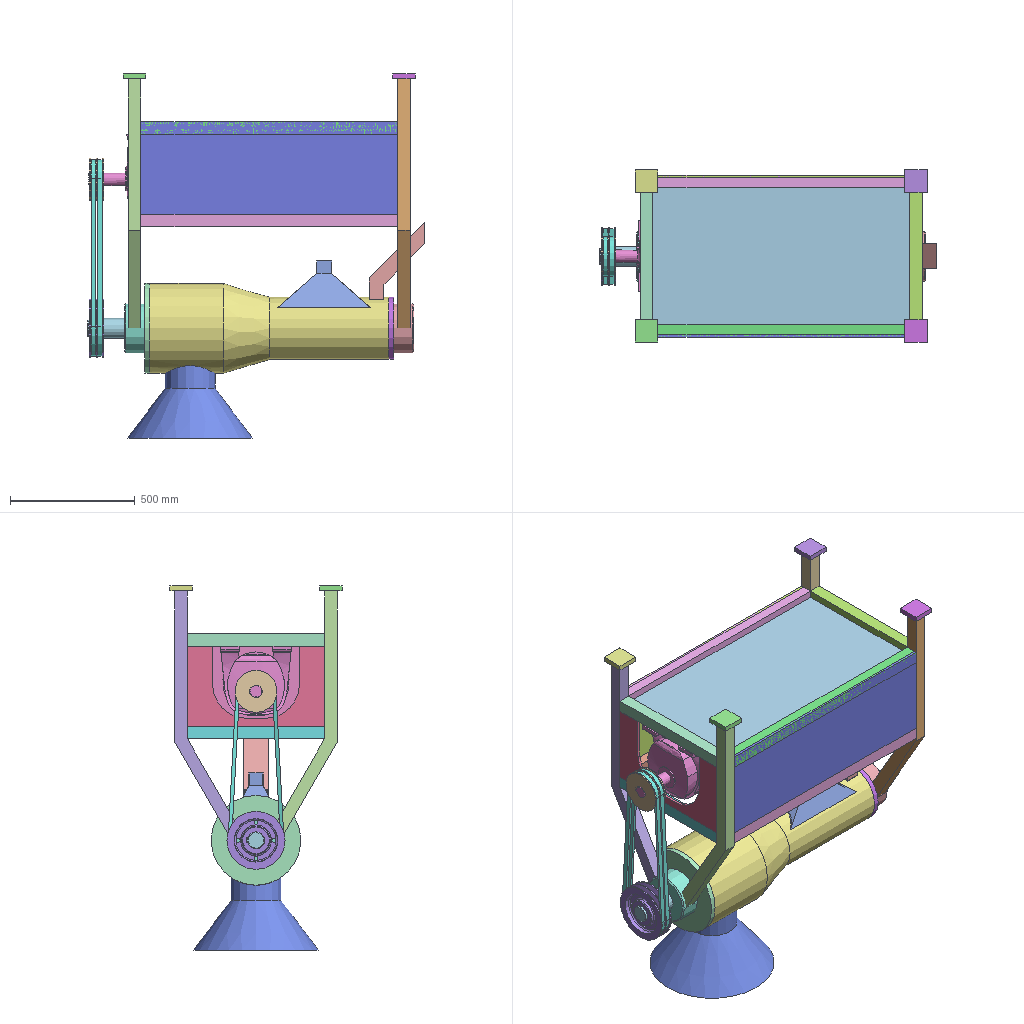Assembly | NX | 16 different items | 17 placed | box 1349 x 690 x 1460 mm
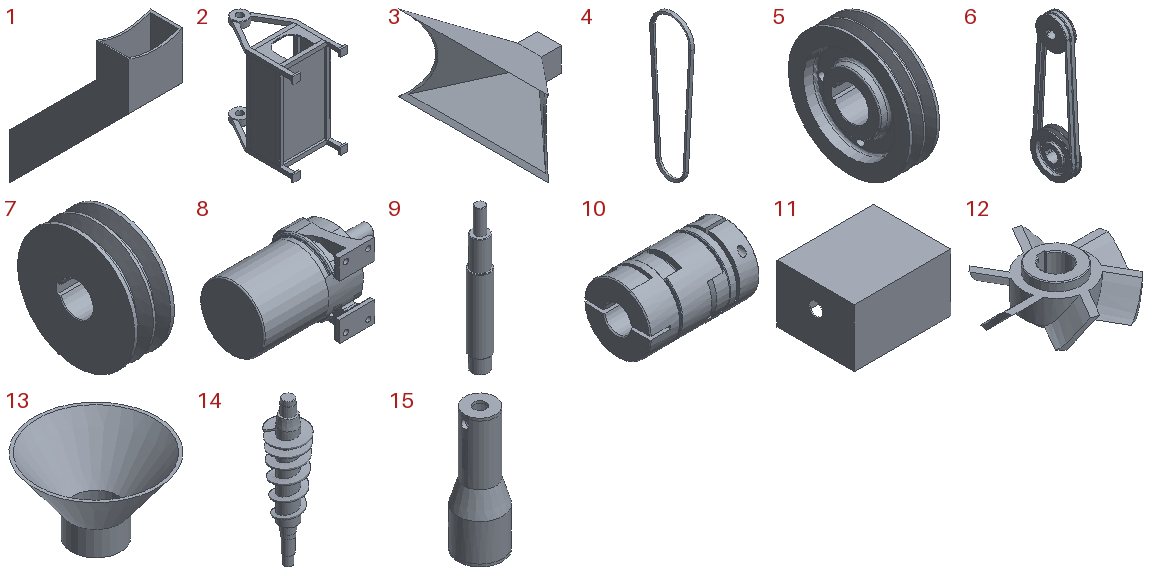Parts list (item | name | quantity | parent item | size | volume | features):
1 | - | x1 | - | 100 x 220.919 x 308.781 mm | 414084 mm3 | features DATUM_CSYS 3, EXTRUDE 2, SKETCH 2, CHAMFER 1, SHELL 1
2 | - | x1 | - | 690 x 1120 x 1170 mm | 52680048 mm3 | features DATUM_CSYS 11, EXTRUDE 10, SKETCH 10, EXTRACT_BODY 8, Container 2, Geometry Instance 2, LINKED_FACE 2, CHAMFER 1, CYLINDER 1, LINKED_CURVE 1
3 | - | x1 | - | 188.137 x 373.11 x 188.928 mm | 418507 mm3 | features NSIDED_SURFACE 6, DATUM_CSYS 5, LINE 4, SKETCH 3, EXTRUDE 2, SEW 1, SHELL 1
4 | - | x2 | in 6 | 19 x 224 x 789.47 mm | 368031 mm3 | features sk_皮带 2
5 | - | x1 | in 6 | 57.5 x 233.6 x 233.6 mm | 1208197 mm3 | features 大带轮_孔板轮(A) 2
6 | - | x1 | - | 57.5 x 233.6 x 799.07 mm | 2816875 mm3 | features sk_皮带 2, 大带轮_孔板轮(A) 2, 小带轮_实心轮 2
7 | - | x1 | in 6 | 57.5 x 169.6 x 169.6 mm | 872615 mm3 | features 小带轮_实心轮 2
8 | - | x1 | - | 553.467 x 279.469 x 285.867 mm | 20300035 mm3 | features BREP 1
9 | - | x1 | - | 80 x 80 x 580 mm | 2266189 mm3 | features CYLINDER 4, CHAMFER 1, DATUM_CSYS 1
10 | - | x1 | - | 165 x 100 x 100 mm | 960558 mm3 | features BREP 5
11 | - | x1 | - | 500 x 400 x 300 mm | 3606133 mm3 | features DATUM_CSYS 2, BLOCK 1, EXTRUDE 1, SHELL 1, SKETCH 1
12 | - | x1 | - | 300.002 x 290.157 x 100 mm | 1656356 mm3 | features DATUM_CSYS 7, EXTRUDE 7, EXTRACT_BODY 6, SKETCH 6, BLEND 2, CHAMFER 1, Container 1, Geometry Instance 1, HOLE PACKAGE 1, SIMPLE HOLE 1, UNITE 1
13 | - | x1 | - | 500 x 500 x 300 mm | 3245287 mm3 | features CONE 1, CYLINDER 1, DATUM_CSYS 1, SHELL 1
14 | - | x1 | - | 177.285 x 178.372 x 728 mm | 4210187 mm3 | features CYLINDER 7, DATUM_CSYS 4, CHAMFER 2, SKETCH 2, UNITE 2, EXTRUDE 1, HELIX 1, LINE 1, SKIN 1
15 | - | x1 | - | 360 x 360 x 1000 mm | 21575281 mm3 | features CYLINDER 4, DATUM_CSYS 4, EXTRUDE 3, SKETCH 3, SPLIT BODY 2, CHAMFER 1, SHELL 1
16 | Fruit Pulper General Assembly | x1 | - | - | - | -
Mates (type | each side: item.copy, entity, surface, feature):
Touch | 12.1 face cylinder Ø67 Hole(14) | 5.1 face cylinder Large Pulley_Web Plate Wheel(A)(1)
Touch | 14.1 face cylinder Cylinder(2) | 12.1 face cylinder Extrude(13)
Touch | 15.1 face cylinder Cylinder(1) | 14.1 face cylinder Cylinder(7)
Distance | 15.1 face plane Cylinder(1) | 14.1 face plane Cylinder(4)
Touch | 9.1 face cylinder Cylinder(2) | 5.1 face cylinder Large Pulley_Web Plate Wheel(A)(1)
Distance | 9.1 face plane Cylinder(3) | 5.1 face plane Large Pulley_Web Plate Wheel(A)(1)
Touch | 10.1 face cylinder Body(0) | 9.1 face cylinder Cylinder(5)
Distance | 10.1 face plane Body(0) | 14.1 face plane Cylinder(2)
Distance | 12.1 face plane Extrude(1) | 9.1 face plane Cylinder(3)
Distance | 8.1 face plane Body(0) | 7.1 face plane Small Pulley_Solid Wheel(1)
Touch | 7.1 face cylinder Small Pulley_Solid Wheel(1) | 8.1 face cylinder Body(0)
Touch | 2.1 face plane Extrude(2) | 15.1 face plane Cylinder(2)
Touch | 2.1 face cylinder Cylinder(3) | 9.1 face cylinder Cylinder(3)
Center12 | 12.1 face plane Extrude(1) | 12.1 face plane Extrude(1) | 13.1 face cylinder Shell(4)
Distance | 13.1 face plane Cylinder(2) | 12.1 face cylinder Ø67 Hole(14)
Center12 | 3.1 face plane Extrude(15) | 3.1 face plane Extrude(15) | 15.1 face cylinder Cylinder(1)
Touch | 3.1 face cylinder Extrude(17) | 15.1 face cylinder Cylinder(1)
Center22 | 3.1 face plane Extrude(15) | 3.1 face plane Extrude(15) | 15.1 face plane Extrude(10) | 15.1 face plane Extrude(10)
Touch | 13.1 face cylinder Shell(4) | 15.1 face cylinder Extrude(9)
Center12 | 1.1 face plane Extrude(1) | 1.1 face plane Extrude(1) | 15.1 face cylinder Extrude(11) | 2 times
Touch | 1.1 face cylinder Extrude(4) | 15.1 face cylinder Cylinder(1)